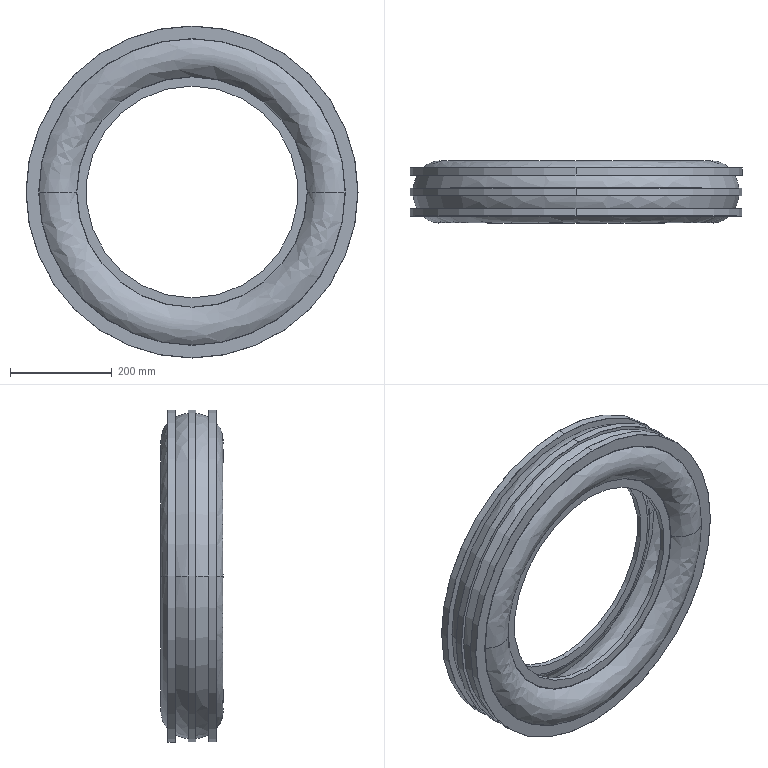Part | SolidWorks | 1 solid | 60 faces | box 652 x 122 x 652 mm | volume 6413789 mm3 | torus 24 | spline 16 | cylinder 10 | plane 10 | commonest cylinder face diameters 652 x6 416 x4